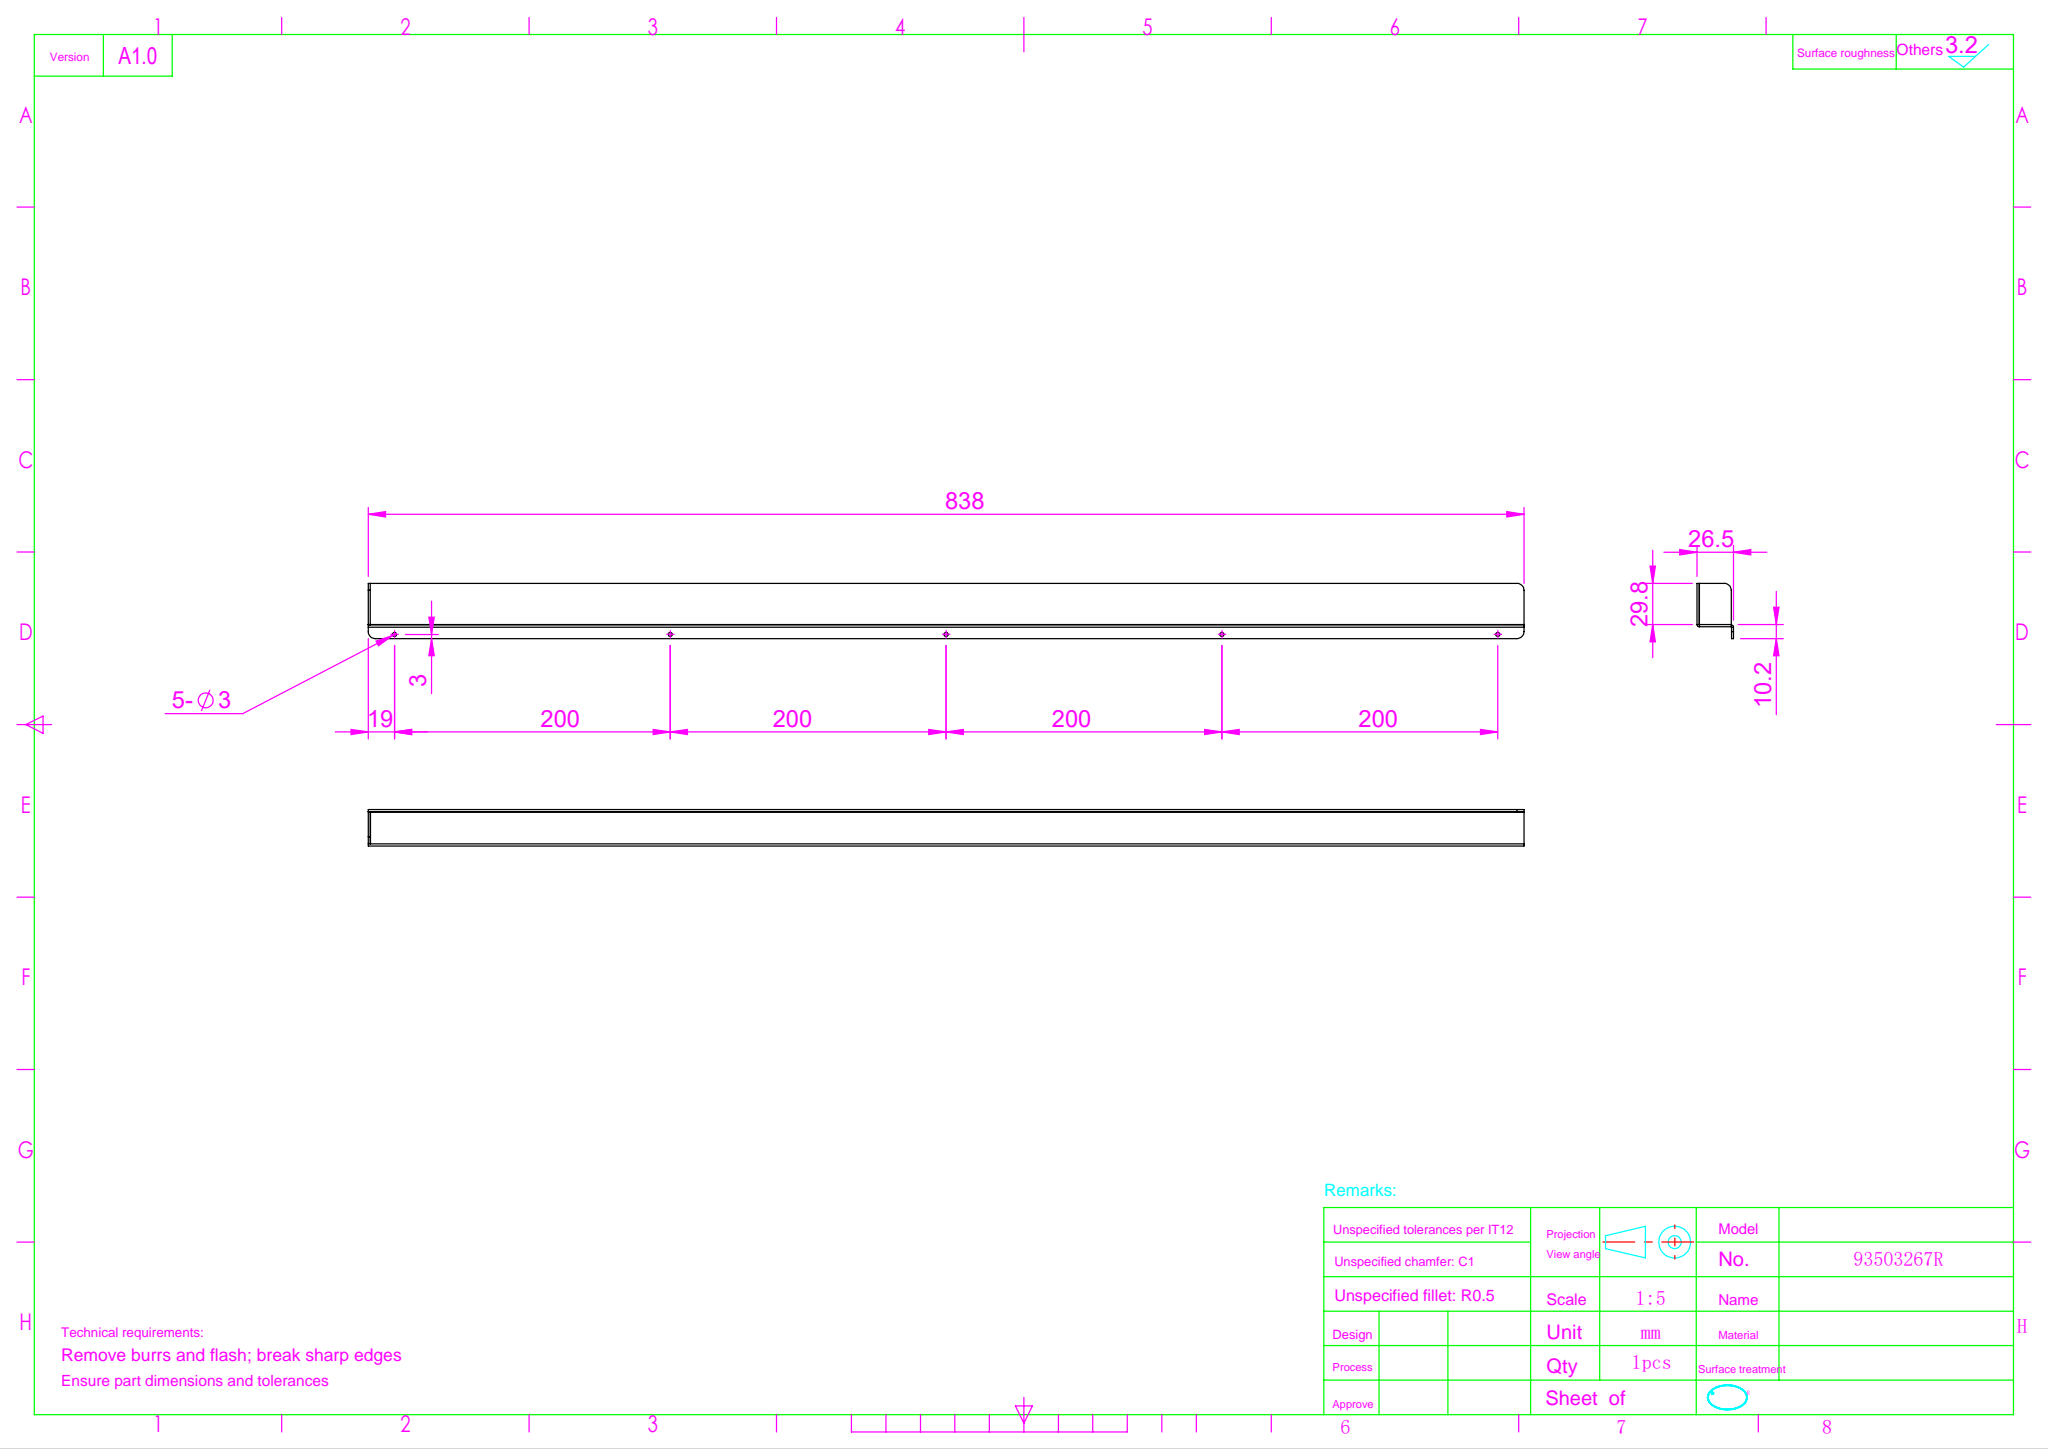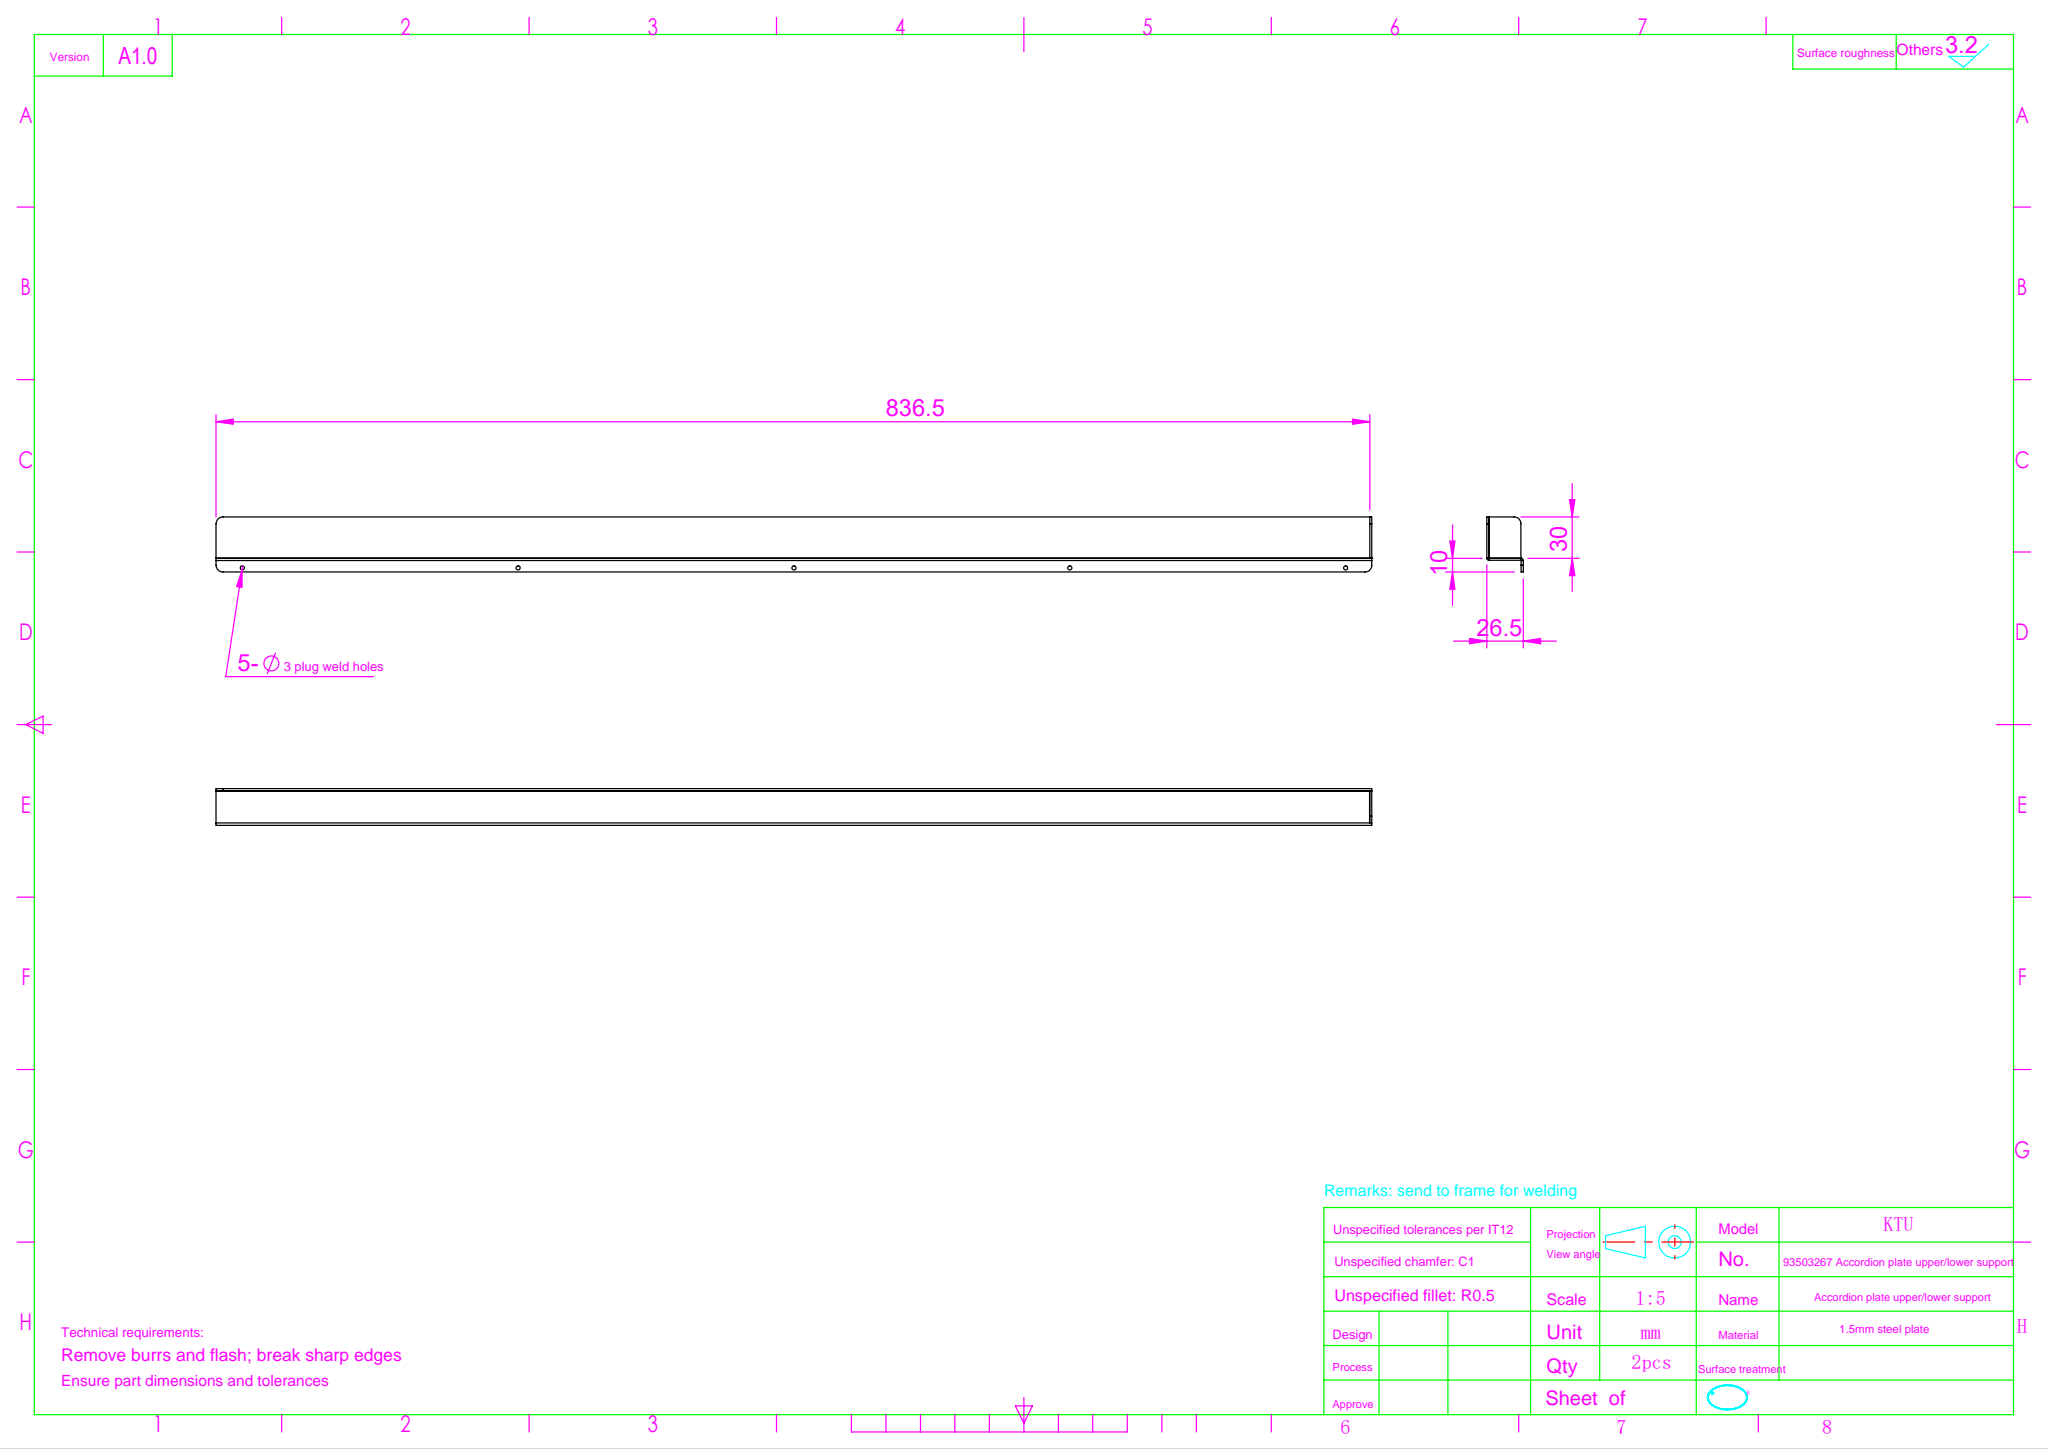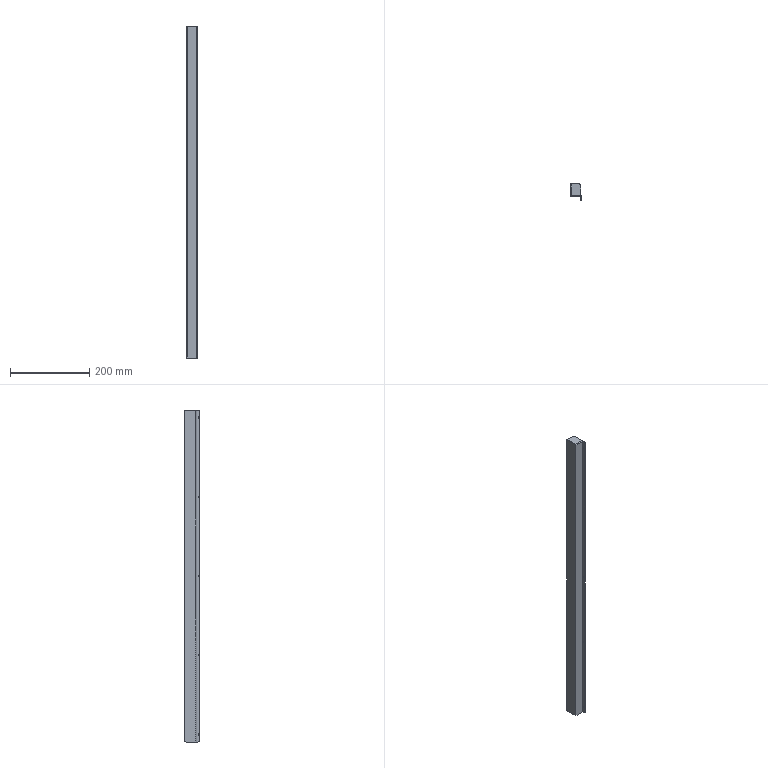Part | SolidWorks | features MirrorStock 1 | 1 solid | 46 faces | box 26.5 x 40 x 838 mm | volume 81620 mm3 | plane 26 | cylinder 20 | commonest cylinder face diameters 3 x10 10 x4 0.4 x3 3.4 x3